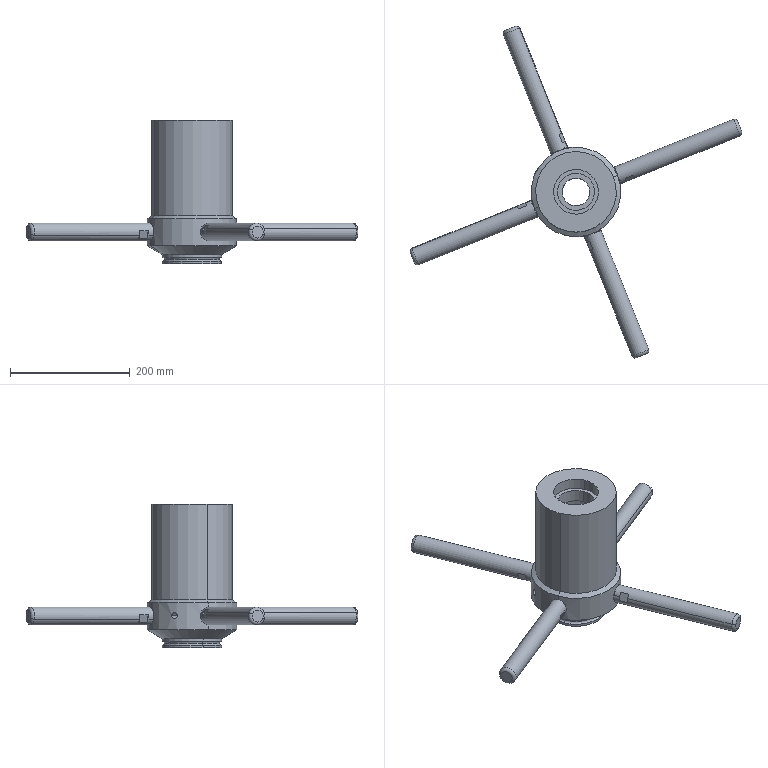Part | SolidWorks | features BaseBody 5 | 5 solids | 119 faces | box 555.753 x 555.753 x 240 mm | volume 3106019 mm3 | plane 45 | cylinder 42 | cone 20 | torus 12 | commonest cylinder face diameters 26 x16 30 x8 100 x4 10 x2 46 x2 62 x2